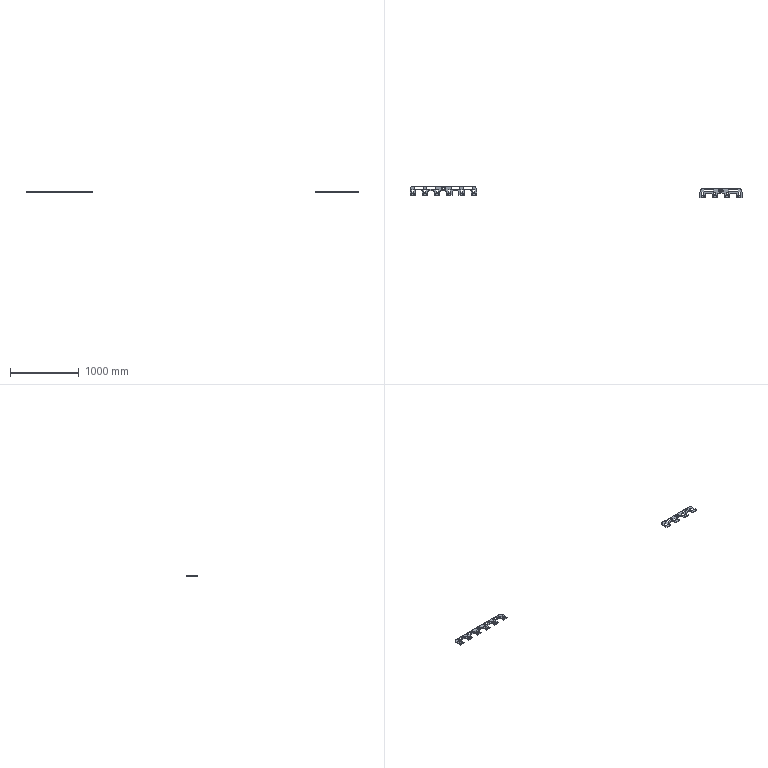NC program | NX | posted with a generic post | part box 4825 x 168.213 x 13 mm
Lines 4013 to 4378 of 4378:
(PLANAR_MILL_COPY_1_COPY , TOOL : D6A45)
N7976 T07 M6
N7978 G54
N7980 G17 G0 G90 X431.6 Y-35.73 S9500 M3
N7982 G43 Z30. H7
N7984 Z0.
N7986 G94 G1 Z-1. F1400.
N7988 X430.9 Y-36.134
N7990 G3 X430.4 Y-37. R1.
N7992 G1 Y-54.
N7994 G3 X432.5 Y-56.1 R2.1
N7996 G1 X456.5
N7998 G3 X458.6 Y-54. R2.1
N8000 G1 Y-20.
N8002 G3 X456.5 Y-17.9 R2.1
N8004 G1 X432.5
N8006 G3 X430.4 Y-20. R2.1
N8008 G1 Y-37.
N8010 G3 X430.9 Y-37.866 R1.
N8012 G1 X431.6 Y-38.27
N8014 Z0.
N8016 G0 Z30.
N8018 X356.87 Y21.9
N8020 Z0.
N8022 G1 Z-1.
N8024 X356.466 Y22.6
N8026 G3 X355.6 Y23.1 R1.
N8028 G1 X294.7
N8030 G3 X292.6 Y21. R2.1
N8032 G1 Y-5.
N8034 G3 X294.7 Y-7.1 R2.1
N8036 G1 X416.5
N8038 G3 X418.6 Y-5. R2.1
N8040 G1 Y21.
N8042 G3 X416.5 Y23.1 R2.1
N8044 G1 X355.6
N8046 G3 X354.734 Y22.6 R1.
N8048 G1 X354.33 Y21.9
N8050 Z0.
N8052 G0 Z30.
N8054 X87.875 Y36.1
N8056 Z0.
N8058 G1 Z-1.
N8060 X88.279 Y35.4
N8062 G3 X89.145 Y34.9 R1.
N8064 G1 X433.4
N8066 G2 X484.3 Y-16. R50.9
N8068 G1 Y-66.3
N8070 G2 X483.3 Y-67.3 R1.
N8072 G1 X405.7
N8074 G2 X404.7 Y-66.3 R1.
N8076 G1 Y-38.
N8078 G3 X385.6 Y-18.9 R19.1
N8080 G1 X325.6
N8082 G3 X306.5 Y-38. R19.1
N8084 G1 Y-66.3
N8086 G2 X305.5 Y-67.3 R1.
N8088 G1 X227.9
N8090 G2 X226.9 Y-66.3 R1.
N8092 G1 Y-53.95
N8094 G3 X207.8 Y-34.85 R19.1
N8096 G1 X147.8
N8098 G3 X128.7 Y-53.95 R19.1
N8100 G1 Y-66.3
N8102 G2 X127.7 Y-67.3 R1.
N8104 G1 X86.428
N8106 G3 X85.562 Y-67.8 R1.
N8108 G1 X85.158 Y-68.5
N8110 Z0.
N8112 G0 Z30.
N8114 X279.6 Y-38.27
N8116 Z0.
N8118 G1 Z-1.
N8120 X280.3 Y-37.866
N8122 G3 X280.8 Y-37. R1.
N8124 G1 Y-20.
N8126 G3 X278.7 Y-17.9 R2.1
N8128 G1 X254.7
N8130 G3 X252.6 Y-20. R2.1
N8132 G1 Y-54.
N8134 G3 X254.7 Y-56.1 R2.1
N8136 G1 X278.7
N8138 G3 X280.8 Y-54. R2.1
N8140 G1 Y-37.
N8142 G3 X280.3 Y-36.134 R1.
N8144 G1 X279.6 Y-35.73
N8146 Z0.
N8148 G0 Z30.
N8150 X179.07 Y21.9
N8152 Z0.
N8154 G1 Z-1.
N8156 X178.666 Y22.6
N8158 G3 X177.8 Y23.1 R1.
N8160 G1 X116.9
N8162 G3 X114.8 Y21. R2.1
N8164 G1 Y-5.
N8166 G3 X116.9 Y-7.1 R2.1
N8168 G1 X238.7
N8170 G3 X240.8 Y-5. R2.1
N8172 G1 Y21.
N8174 G3 X238.7 Y23.1 R2.1
N8176 G1 X177.8
N8178 G3 X176.934 Y22.6 R1.
N8180 G1 X176.53 Y21.9
N8182 Z0.
N8184 G0 Z30.
N8186 X85.456 Y-54.9
N8188 Z0.
N8190 G1 Z-1.
N8192 X85.86 Y-55.6
N8194 G3 X86.726 Y-56.1 R1.
N8196 G1 X100.9
N8198 G3 X103. Y-54. R2.1
N8200 G1 Y-20.
N8202 G3 X100.9 Y-17.9 R2.1
N8204 G1 X87.741
N8206 G3 X86.875 Y-18.4 R1.
N8208 G1 X86.471 Y-19.1
N8210 Z0.
N8212 G0 Z30.
(PLANAR_MILL_COPY_COPY_COPY , TOOL : D6A45)
N8214 X464.012 Y-95.242
N8216 Z-3.
N8218 G1 Z-4.
N8220 X463.634 Y-96.05
N8222 G3 X464.5 Y-96.55 R1.
N8224 X466.85 Y-94.2 R2.35
N8226 X464.5 Y-96.55 R-2.35
N8228 X465.366 Y-96.05 R1.
N8230 G1 X464.988 Y-95.242
N8232 Z-3.
N8234 G0 Z30.
N8236 X464.493 Y-71.1
N8238 Z-3.
N8240 G1 Z-4.
N8242 Y-70.056
N8244 G3 X464.018 Y-69.9 R0.5
N8246 X464.982 Y-69.9 R-2.35
N8248 X464.507 Y-70.056 R0.5
N8250 G1 Y-71.1
N8252 Z-3.
N8254 G0 Z30.
N8256 X424.493
N8258 Z-3.
N8260 G1 Z-4.
N8262 Y-70.056
N8264 G3 X424.018 Y-69.9 R0.5
N8266 X424.982 Y-69.9 R-2.35
N8268 X424.507 Y-70.056 R0.5
N8270 G1 Y-71.1
N8272 Z-3.
N8274 G0 Z30.
N8276 X424.012 Y-95.242
N8278 Z-3.
N8280 G1 Z-4.
N8282 X423.634 Y-96.05
N8284 G3 X424.5 Y-96.55 R1.
N8286 X426.85 Y-94.2 R2.35
N8288 X424.5 Y-96.55 R-2.35
N8290 X425.366 Y-96.05 R1.
N8292 G1 X424.988 Y-95.242
N8294 Z-3.
N8296 G0 Z30.
N8298 X286.212
N8300 Z-3.
N8302 G1 Z-4.
N8304 X285.834 Y-96.05
N8306 G3 X286.7 Y-96.55 R1.
N8308 X289.05 Y-94.2 R2.35
N8310 X286.7 Y-96.55 R-2.35
N8312 X287.566 Y-96.05 R1.
N8314 G1 X287.188 Y-95.242
N8316 Z-3.
N8318 G0 Z30.
N8320 X286.693 Y-71.1
N8322 Z-3.
N8324 G1 Z-4.
N8326 Y-70.056
N8328 G3 X286.218 Y-69.9 R0.5
N8330 X287.182 Y-69.9 R-2.35
N8332 X286.707 Y-70.056 R0.5
N8334 G1 Y-71.1
N8336 Z-3.
N8338 G0 Z30.
N8340 X246.693
N8342 Z-3.
N8344 G1 Z-4.
N8346 Y-70.056
N8348 G3 X246.218 Y-69.9 R0.5
N8350 X247.182 Y-69.9 R-2.35
N8352 X246.707 Y-70.056 R0.5
N8354 G1 Y-71.1
N8356 Z-3.
N8358 G0 Z30.
N8360 X246.212 Y-95.242
N8362 Z-3.
N8364 G1 Z-4.
N8366 X245.834 Y-96.05
N8368 G3 X246.7 Y-96.55 R1.
N8370 X249.05 Y-94.2 R2.35
N8372 X246.7 Y-96.55 R-2.35
N8374 X247.566 Y-96.05 R1.
N8376 G1 X247.188 Y-95.242
N8378 Z-3.
N8380 G0 Z30.
N8382 X307.913 Y-70.492
N8384 Z-3.
N8386 G1 Z-4.
N8388 X307.465 Y-70.043
N8390 G3 X306.5 Y-69.782 R1.
N8392 G1 Y-99.9
N8394 G2 X305.5 Y-100.9 R1.
N8396 G1 X227.9
N8398 G2 X226.9 Y-99.9 R1.
N8400 G1 Y-69.782
N8402 G3 X225.935 Y-70.043 R1.
N8404 G1 X225.487 Y-70.492
N8406 Z-3.
N8408 G0 Z30.
N8410 X485.713
N8412 Z-3.
N8414 G1 Z-4.
N8416 X485.265 Y-70.043
N8418 G3 X484.3 Y-69.782 R1.
N8420 G1 Y-99.9
N8422 G2 X483.3 Y-100.9 R1.
N8424 G1 X405.7
N8426 G2 X404.7 Y-99.9 R1.
N8428 G1 Y-69.782
N8430 G3 X403.735 Y-70.043 R1.
N8432 G1 X403.287 Y-70.492
N8434 Z-3.
N8436 G0 Z30.
N8438 M5
(ZLEVEL_PROFILE_COPY_3_COPY_COPY , TOOL : D10)
N8440 T10 M6
N8442 G54
N8444 G17 G0 G90 X105.202 Y42.5 S9500 M3
N8446 G43 Z30. H10
N8448 Z-7.525
N8450 G94 G1 Z-12.525 F1000.
N8452 X106.934 Y39.5
N8454 G3 X107.8 Y39. R1.
N8456 G1 X433.4 F1200.
N8458 G2 X488.4 Y-16. R55.
N8460 G1 Y-100.
N8462 G2 X483.4 Y-105. R5.
N8464 G1 X405.6
N8466 G2 X400.6 Y-100. R5.
N8468 G1 Y-38.
N8470 G3 X385.6 Y-23. R15.
N8472 G1 X325.6
N8474 G3 X310.6 Y-38. R15.
N8476 G1 Y-100.
N8478 G2 X305.6 Y-105. R5.
N8480 G1 X227.8
N8482 G2 X222.8 Y-100. R5.
N8484 G1 Y-53.95
N8486 G3 X207.8 Y-38.95 R15.
N8488 G1 X147.8
N8490 G3 X132.8 Y-53.95 R15.
N8492 G1 Y-100.
N8494 G2 X127.8 Y-105. R5.
N8496 G1 X107.8
N8498 G3 X106.934 Y-105.5 R1.
N8500 G1 X105.202 Y-108.5
N8502 Z-7.525
N8504 G0 Z30.
N8506 Y42.5
N8508 Z-7.65
N8510 G1 Z-12.65 F1000.
N8512 X106.934 Y39.5
N8514 G3 X107.8 Y39. R1.
N8516 G1 X433.4 F1200.
N8518 G2 X488.4 Y-16. R55.
N8520 G1 Y-100.
N8522 G2 X483.4 Y-105. R5.
N8524 G1 X405.6
N8526 G2 X400.6 Y-100. R5.
N8528 G1 Y-38.
N8530 G3 X385.6 Y-23. R15.
N8532 G1 X325.6
N8534 G3 X310.6 Y-38. R15.
N8536 G1 Y-100.
N8538 G2 X305.6 Y-105. R5.
N8540 G1 X227.8
N8542 G2 X222.8 Y-100. R5.
N8544 G1 Y-53.95
N8546 G3 X207.8 Y-38.95 R15.
N8548 G1 X147.8
N8550 G3 X132.8 Y-53.95 R15.
N8552 G1 Y-100.
N8554 G2 X127.8 Y-105. R5.
N8556 G1 X107.8
N8558 G3 X106.934 Y-105.5 R1.
N8560 G1 X105.202 Y-108.5
N8562 Z-7.65
N8564 G0 Z30.
N8566 Y42.5
N8568 Z-7.775
N8570 G1 Z-12.775 F1000.
N8572 X106.934 Y39.5
N8574 G3 X107.8 Y39. R1.
N8576 G1 X433.4 F1200.
N8578 G2 X488.4 Y-16. R55.
N8580 G1 Y-100.
N8582 G2 X483.4 Y-105. R5.
N8584 G1 X405.6
N8586 G2 X400.6 Y-100. R5.
N8588 G1 Y-38.
N8590 G3 X385.6 Y-23. R15.
N8592 G1 X325.6
N8594 G3 X310.6 Y-38. R15.
N8596 G1 Y-100.
N8598 G2 X305.6 Y-105. R5.
N8600 G1 X227.8
N8602 G2 X222.8 Y-100. R5.
N8604 G1 Y-53.95
N8606 G3 X207.8 Y-38.95 R15.
N8608 G1 X147.8
N8610 G3 X132.8 Y-53.95 R15.
N8612 G1 Y-100.
N8614 G2 X127.8 Y-105. R5.
N8616 G1 X107.8
N8618 G3 X106.934 Y-105.5 R1.
N8620 G1 X105.202 Y-108.5
N8622 Z-7.775
N8624 G0 Z30.
N8626 Y42.5
N8628 Z-7.9
N8630 G1 Z-12.9 F1000.
N8632 X106.934 Y39.5
N8634 G3 X107.8 Y39. R1.
N8636 G1 X433.4 F1200.
N8638 G2 X488.4 Y-16. R55.
N8640 G1 Y-100.
N8642 G2 X483.4 Y-105. R5.
N8644 G1 X405.6
N8646 G2 X400.6 Y-100. R5.
N8648 G1 Y-38.
N8650 G3 X385.6 Y-23. R15.
N8652 G1 X325.6
N8654 G3 X310.6 Y-38. R15.
N8656 G1 Y-100.
N8658 G2 X305.6 Y-105. R5.
N8660 G1 X227.8
N8662 G2 X222.8 Y-100. R5.
N8664 G1 Y-53.95
N8666 G3 X207.8 Y-38.95 R15.
N8668 G1 X147.8
N8670 G3 X132.8 Y-53.95 R15.
N8672 G1 Y-100.
N8674 G2 X127.8 Y-105. R5.
N8676 G1 X107.8
N8678 G3 X106.934 Y-105.5 R1.
N8680 G1 X105.202 Y-108.5
N8682 Z-7.9
N8684 G0 Z30.
N8686 M5
N8688 M2